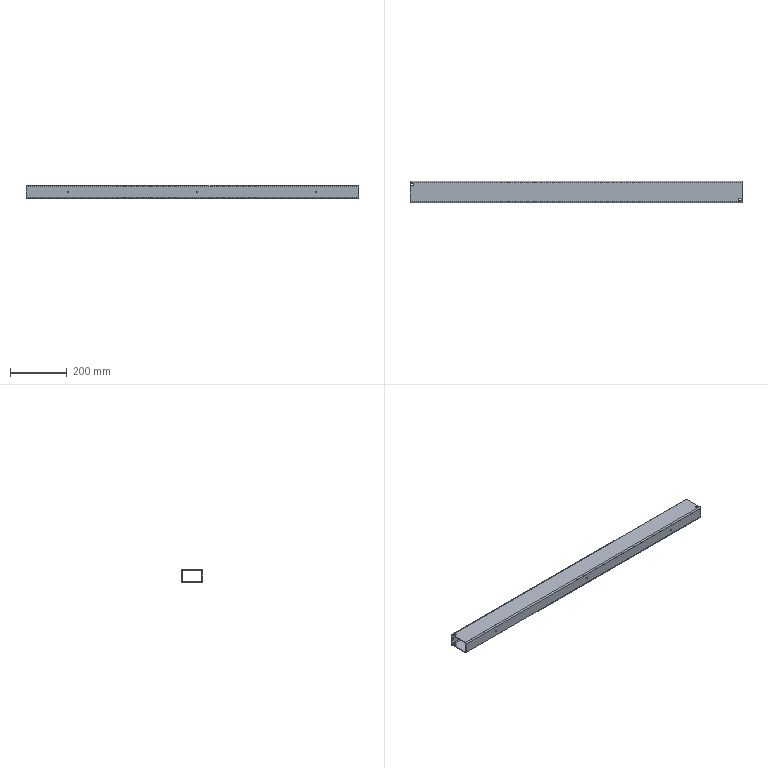Part | STEP file | [03]-3 | 1 solid | 42 faces | box 1175 x 75 x 45 mm | volume 605779 mm3 | cylinder 32 | plane 10 | commonest cylinder face diameters 10 x12 4 x6 12 x6 4.6 x4 9.2 x4
STEP:
#1=CARTESIAN_POINT('',(149.5,0.,20.5));
#2=VERTEX_POINT('',#1);
#3=CARTESIAN_POINT('',(149.5,0.,24.5));
#4=VERTEX_POINT('',#3);
#5=CARTESIAN_POINT('',(149.5,0.,22.5));
#6=DIRECTION('',(0.,1.,0.));
#7=DIRECTION('',(0.,0.,1.));
#8=AXIS2_PLACEMENT_3D('',#5,#6,#7);
#9=CIRCLE('',#8,2.);
#10=EDGE_CURVE('',#2,#4,#9,.T.);
#11=ORIENTED_EDGE('',*,*,#10,.F.);
#12=CARTESIAN_POINT('',(149.5,2.3,20.5));
#13=VERTEX_POINT('',#12);
#14=CARTESIAN_POINT('',(149.5,0.,20.5));
#15=DIRECTION('',(0.,1.,0.));
#16=VECTOR('',#15,1000.);
#17=LINE('',#14,#16);
#18=EDGE_CURVE('',#2,#13,#17,.T.);
#19=ORIENTED_EDGE('',*,*,#18,.T.);
#20=CARTESIAN_POINT('',(149.5,2.3,24.5));
#21=VERTEX_POINT('',#20);
#22=CARTESIAN_POINT('',(149.5,2.3,22.5));
#23=DIRECTION('',(0.,-1.,0.));
#24=DIRECTION('',(0.,0.,-1.));
#25=AXIS2_PLACEMENT_3D('',#22,#23,#24);
#26=CIRCLE('',#25,2.);
#27=EDGE_CURVE('',#21,#13,#26,.T.);
#28=ORIENTED_EDGE('',*,*,#27,.F.);
#29=CARTESIAN_POINT('',(149.5,0.,24.5));
#30=DIRECTION('',(0.,1.,0.));
#31=VECTOR('',#30,1000.);
#32=LINE('',#29,#31);
#33=EDGE_CURVE('',#4,#21,#32,.T.);
#34=ORIENTED_EDGE('',*,*,#33,.F.);
#35=EDGE_LOOP('',(#11,#19,#28,#34));
#36=FACE_OUTER_BOUND('',#35,.T.);
#37=CARTESIAN_POINT('',(149.5,0.,22.5));
#38=DIRECTION('',(0.,1.,0.));
#39=DIRECTION('',(0.,0.,1.));
#40=AXIS2_PLACEMENT_3D('',#37,#38,#39);
#41=CYLINDRICAL_SURFACE('',#40,2.);
#42=ADVANCED_FACE('',(#36),#41,.F.);
#43=CARTESIAN_POINT('',(604.5,0.,20.5));
#44=VERTEX_POINT('',#43);
#45=CARTESIAN_POINT('',(604.5,0.,24.5));
#46=VERTEX_POINT('',#45);
#47=CARTESIAN_POINT('',(604.5,0.,22.5));
#48=DIRECTION('',(0.,1.,0.));
#49=DIRECTION('',(0.,0.,1.));
#50=AXIS2_PLACEMENT_3D('',#47,#48,#49);
#51=CIRCLE('',#50,2.);
#52=EDGE_CURVE('',#44,#46,#51,.T.);
#53=ORIENTED_EDGE('',*,*,#52,.F.);
#54=CARTESIAN_POINT('',(604.5,2.3,20.5));
#55=VERTEX_POINT('',#54);
#56=CARTESIAN_POINT('',(604.5,0.,20.5));
#57=DIRECTION('',(0.,1.,0.));
#58=VECTOR('',#57,1000.);
#59=LINE('',#56,#58);
#60=EDGE_CURVE('',#44,#55,#59,.T.);
#61=ORIENTED_EDGE('',*,*,#60,.T.);
#62=CARTESIAN_POINT('',(604.5,2.3,24.5));
#63=VERTEX_POINT('',#62);
#64=CARTESIAN_POINT('',(604.5,2.3,22.5));
#65=DIRECTION('',(0.,-1.,0.));
#66=DIRECTION('',(0.,0.,-1.));
#67=AXIS2_PLACEMENT_3D('',#64,#65,#66);
#68=CIRCLE('',#67,2.);
#69=EDGE_CURVE('',#63,#55,#68,.T.);
#70=ORIENTED_EDGE('',*,*,#69,.F.);
#71=CARTESIAN_POINT('',(604.5,0.,24.5));
#72=DIRECTION('',(0.,1.,0.));
#73=VECTOR('',#72,1000.);
#74=LINE('',#71,#73);
#75=EDGE_CURVE('',#46,#63,#74,.T.);
#76=ORIENTED_EDGE('',*,*,#75,.F.);
#77=EDGE_LOOP('',(#53,#61,#70,#76));
#78=FACE_OUTER_BOUND('',#77,.T.);
#79=CARTESIAN_POINT('',(604.5,0.,22.5));
#80=DIRECTION('',(0.,1.,0.));
#81=DIRECTION('',(0.,0.,1.));
#82=AXIS2_PLACEMENT_3D('',#79,#80,#81);
#83=CYLINDRICAL_SURFACE('',#82,2.);
#84=ADVANCED_FACE('',(#78),#83,.F.);
#85=CARTESIAN_POINT('',(1024.5,0.,20.5));
#86=VERTEX_POINT('',#85);
#87=CARTESIAN_POINT('',(1024.5,0.,24.5));
#88=VERTEX_POINT('',#87);
#89=CARTESIAN_POINT('',(1024.5,0.,22.5));
#90=DIRECTION('',(0.,1.,0.));
#91=DIRECTION('',(0.,0.,1.));
#92=AXIS2_PLACEMENT_3D('',#89,#90,#91);
#93=CIRCLE('',#92,2.);
#94=EDGE_CURVE('',#86,#88,#93,.T.);
#95=ORIENTED_EDGE('',*,*,#94,.F.);
#96=CARTESIAN_POINT('',(1024.5,2.3,20.5));
#97=VERTEX_POINT('',#96);
#98=CARTESIAN_POINT('',(1024.5,0.,20.5));
#99=DIRECTION('',(0.,1.,0.));
#100=VECTOR('',#99,1000.);
#101=LINE('',#98,#100);
#102=EDGE_CURVE('',#86,#97,#101,.T.);
#103=ORIENTED_EDGE('',*,*,#102,.T.);
#104=CARTESIAN_POINT('',(1024.5,2.3,24.5));
#105=VERTEX_POINT('',#104);
#106=CARTESIAN_POINT('',(1024.5,2.3,22.5));
#107=DIRECTION('',(0.,-1.,0.));
#108=DIRECTION('',(0.,0.,-1.));
#109=AXIS2_PLACEMENT_3D('',#106,#107,#108);
#110=CIRCLE('',#109,2.);
#111=EDGE_CURVE('',#105,#97,#110,.T.);
#112=ORIENTED_EDGE('',*,*,#111,.F.);
#113=CARTESIAN_POINT('',(1024.5,0.,24.5));
#114=DIRECTION('',(0.,1.,0.));
#115=VECTOR('',#114,1000.);
#116=LINE('',#113,#115);
#117=EDGE_CURVE('',#88,#105,#116,.T.);
#118=ORIENTED_EDGE('',*,*,#117,.F.);
#119=EDGE_LOOP('',(#95,#103,#112,#118));
#120=FACE_OUTER_BOUND('',#119,.T.);
#121=CARTESIAN_POINT('',(1024.5,0.,22.5));
#122=DIRECTION('',(0.,1.,0.));
#123=DIRECTION('',(0.,0.,1.));
#124=AXIS2_PLACEMENT_3D('',#121,#122,#123);
#125=CYLINDRICAL_SURFACE('',#124,2.);
#126=ADVANCED_FACE('',(#120),#125,.F.);
#127=CARTESIAN_POINT('',(1167.5,75.,27.5));
#128=VERTEX_POINT('',#127);
#129=CARTESIAN_POINT('',(1167.5,75.,17.5));
#130=VERTEX_POINT('',#129);
#131=CARTESIAN_POINT('',(1167.5,75.,22.5));
#132=DIRECTION('',(0.,-1.,0.));
#133=DIRECTION('',(0.,0.,-1.));
#134=AXIS2_PLACEMENT_3D('',#131,#132,#133);
#135=CIRCLE('',#134,5.);
#136=EDGE_CURVE('',#128,#130,#135,.T.);
#137=ORIENTED_EDGE('',*,*,#136,.F.);
#138=CARTESIAN_POINT('',(1167.5,72.7,27.5));
#139=VERTEX_POINT('',#138);
#140=CARTESIAN_POINT('',(1167.5,75.,27.5));
#141=DIRECTION('',(0.,-1.,0.));
#142=VECTOR('',#141,1000.);
#143=LINE('',#140,#142);
#144=EDGE_CURVE('',#128,#139,#143,.T.);
#145=ORIENTED_EDGE('',*,*,#144,.T.);
#146=CARTESIAN_POINT('',(1167.5,72.7,17.5));
#147=VERTEX_POINT('',#146);
#148=CARTESIAN_POINT('',(1167.5,72.7,22.5));
#149=DIRECTION('',(0.,1.,0.));
#150=DIRECTION('',(0.,0.,1.));
#151=AXIS2_PLACEMENT_3D('',#148,#149,#150);
#152=CIRCLE('',#151,5.);
#153=EDGE_CURVE('',#147,#139,#152,.T.);
#154=ORIENTED_EDGE('',*,*,#153,.F.);
#155=CARTESIAN_POINT('',(1167.5,75.,17.5));
#156=DIRECTION('',(0.,-1.,0.));
#157=VECTOR('',#156,1000.);
#158=LINE('',#155,#157);
#159=EDGE_CURVE('',#130,#147,#158,.T.);
#160=ORIENTED_EDGE('',*,*,#159,.F.);
#161=EDGE_LOOP('',(#137,#145,#154,#160));
#162=FACE_OUTER_BOUND('',#161,.T.);
#163=CARTESIAN_POINT('',(1167.5,75.,22.5));
#164=DIRECTION('',(0.,-1.,0.));
#165=DIRECTION('',(0.,0.,-1.));
#166=AXIS2_PLACEMENT_3D('',#163,#164,#165);
#167=CYLINDRICAL_SURFACE('',#166,5.);
#168=ADVANCED_FACE('',(#162),#167,.F.);
#169=CARTESIAN_POINT('',(6.5,75.,27.5));
#170=VERTEX_POINT('',#169);
#171=CARTESIAN_POINT('',(6.5,75.,17.5));
#172=VERTEX_POINT('',#171);
#173=CARTESIAN_POINT('',(6.5,75.,22.5));
#174=DIRECTION('',(0.,-1.,0.));
#175=DIRECTION('',(0.,0.,-1.));
#176=AXIS2_PLACEMENT_3D('',#173,#174,#175);
#177=CIRCLE('',#176,5.);
#178=EDGE_CURVE('',#170,#172,#177,.T.);
#179=ORIENTED_EDGE('',*,*,#178,.F.);
#180=CARTESIAN_POINT('',(6.5,72.7,27.5));
#181=VERTEX_POINT('',#180);
#182=CARTESIAN_POINT('',(6.5,75.,27.5));
#183=DIRECTION('',(0.,-1.,0.));
#184=VECTOR('',#183,1000.);
#185=LINE('',#182,#184);
#186=EDGE_CURVE('',#170,#181,#185,.T.);
#187=ORIENTED_EDGE('',*,*,#186,.T.);
#188=CARTESIAN_POINT('',(6.5,72.7,17.5));
#189=VERTEX_POINT('',#188);
#190=CARTESIAN_POINT('',(6.5,72.7,22.5));
#191=DIRECTION('',(0.,1.,0.));
#192=DIRECTION('',(0.,0.,1.));
#193=AXIS2_PLACEMENT_3D('',#190,#191,#192);
#194=CIRCLE('',#193,5.);
#195=EDGE_CURVE('',#189,#181,#194,.T.);
#196=ORIENTED_EDGE('',*,*,#195,.F.);
#197=CARTESIAN_POINT('',(6.5,75.,17.5));
#198=DIRECTION('',(0.,-1.,0.));
#199=VECTOR('',#198,1000.);
#200=LINE('',#197,#199);
#201=EDGE_CURVE('',#172,#189,#200,.T.);
#202=ORIENTED_EDGE('',*,*,#201,.F.);
#203=EDGE_LOOP('',(#179,#187,#196,#202));
#204=FACE_OUTER_BOUND('',#203,.T.);
#205=CARTESIAN_POINT('',(6.5,75.,22.5));
#206=DIRECTION('',(0.,-1.,0.));
#207=DIRECTION('',(0.,0.,-1.));
#208=AXIS2_PLACEMENT_3D('',#205,#206,#207);
#209=CYLINDRICAL_SURFACE('',#208,5.);
#210=ADVANCED_FACE('',(#204),#209,.F.);
#211=CARTESIAN_POINT('',(1166.5,15.5,42.7));
#212=VERTEX_POINT('',#211);
#213=CARTESIAN_POINT('',(1166.5,5.5,42.7));
#214=VERTEX_POINT('',#213);
#215=CARTESIAN_POINT('',(1166.5,10.5,42.7));
#216=DIRECTION('',(0.,0.,1.));
#217=DIRECTION('',(0.,-1.,0.));
#218=AXIS2_PLACEMENT_3D('',#215,#216,#217);
#219=CIRCLE('',#218,5.);
#220=EDGE_CURVE('',#212,#214,#219,.T.);
#221=ORIENTED_EDGE('',*,*,#220,.F.);
#222=CARTESIAN_POINT('',(1166.5,15.5,45.));
#223=VERTEX_POINT('',#222);
#224=CARTESIAN_POINT('',(1166.5,15.5,42.7));
#225=DIRECTION('',(0.,0.,1.));
#226=VECTOR('',#225,1000.);
#227=LINE('',#224,#226);
#228=EDGE_CURVE('',#212,#223,#227,.T.);
#229=ORIENTED_EDGE('',*,*,#228,.T.);
#230=CARTESIAN_POINT('',(1166.5,5.5,45.));
#231=VERTEX_POINT('',#230);
#232=CARTESIAN_POINT('',(1166.5,10.5,45.));
#233=DIRECTION('',(0.,0.,-1.));
#234=DIRECTION('',(0.,1.,0.));
#235=AXIS2_PLACEMENT_3D('',#232,#233,#234);
#236=CIRCLE('',#235,5.);
#237=EDGE_CURVE('',#231,#223,#236,.T.);
#238=ORIENTED_EDGE('',*,*,#237,.F.);
#239=CARTESIAN_POINT('',(1166.5,5.5,42.7));
#240=DIRECTION('',(0.,0.,1.));
#241=VECTOR('',#240,1000.);
#242=LINE('',#239,#241);
#243=EDGE_CURVE('',#214,#231,#242,.T.);
#244=ORIENTED_EDGE('',*,*,#243,.F.);
#245=EDGE_LOOP('',(#221,#229,#238,#244));
#246=FACE_OUTER_BOUND('',#245,.T.);
#247=CARTESIAN_POINT('',(1166.5,10.5,42.7));
#248=DIRECTION('',(0.,0.,1.));
#249=DIRECTION('',(0.,-1.,0.));
#250=AXIS2_PLACEMENT_3D('',#247,#248,#249);
#251=CYLINDRICAL_SURFACE('',#250,5.);
#252=ADVANCED_FACE('',(#246),#251,.F.);
#253=CARTESIAN_POINT('',(7.5,59.5,2.3));
#254=VERTEX_POINT('',#253);
#255=CARTESIAN_POINT('',(7.5,69.5,2.3));
#256=VERTEX_POINT('',#255);
#257=CARTESIAN_POINT('',(7.5,64.5,2.3));
#258=DIRECTION('',(0.,0.,-1.));
#259=DIRECTION('',(0.,1.,0.));
#260=AXIS2_PLACEMENT_3D('',#257,#258,#259);
#261=CIRCLE('',#260,5.);
#262=EDGE_CURVE('',#254,#256,#261,.T.);
#263=ORIENTED_EDGE('',*,*,#262,.F.);
#264=CARTESIAN_POINT('',(7.5,59.5,0.));
#265=VERTEX_POINT('',#264);
#266=CARTESIAN_POINT('',(7.5,59.5,2.3));
#267=DIRECTION('',(0.,0.,-1.));
#268=VECTOR('',#267,1000.);
#269=LINE('',#266,#268);
#270=EDGE_CURVE('',#254,#265,#269,.T.);
#271=ORIENTED_EDGE('',*,*,#270,.T.);
#272=CARTESIAN_POINT('',(7.5,69.5,0.));
#273=VERTEX_POINT('',#272);
#274=CARTESIAN_POINT('',(7.5,64.5,0.));
#275=DIRECTION('',(0.,0.,1.));
#276=DIRECTION('',(0.,-1.,0.));
#277=AXIS2_PLACEMENT_3D('',#274,#275,#276);
#278=CIRCLE('',#277,5.);
#279=EDGE_CURVE('',#273,#265,#278,.T.);
#280=ORIENTED_EDGE('',*,*,#279,.F.);
#281=CARTESIAN_POINT('',(7.5,69.5,2.3));
#282=DIRECTION('',(0.,0.,-1.));
#283=VECTOR('',#282,1000.);
#284=LINE('',#281,#283);
#285=EDGE_CURVE('',#256,#273,#284,.T.);
#286=ORIENTED_EDGE('',*,*,#285,.F.);
#287=EDGE_LOOP('',(#263,#271,#280,#286));
#288=FACE_OUTER_BOUND('',#287,.T.);
#289=CARTESIAN_POINT('',(7.5,64.5,2.3));
#290=DIRECTION('',(0.,0.,-1.));
#291=DIRECTION('',(0.,1.,0.));
#292=AXIS2_PLACEMENT_3D('',#289,#290,#291);
#293=CYLINDRICAL_SURFACE('',#292,5.);
#294=ADVANCED_FACE('',(#288),#293,.F.);
#295=CARTESIAN_POINT('',(1024.5,51.,0.));
#296=VERTEX_POINT('',#295);
#297=CARTESIAN_POINT('',(1024.5,39.,0.));
#298=VERTEX_POINT('',#297);
#299=CARTESIAN_POINT('',(1024.5,45.,0.));
#300=DIRECTION('',(0.,0.,1.));
#301=DIRECTION('',(0.,-1.,0.));
#302=AXIS2_PLACEMENT_3D('',#299,#300,#301);
#303=CIRCLE('',#302,6.);
#304=EDGE_CURVE('',#296,#298,#303,.T.);
#305=ORIENTED_EDGE('',*,*,#304,.F.);
#306=CARTESIAN_POINT('',(1024.5,51.,2.3));
#307=VERTEX_POINT('',#306);
#308=CARTESIAN_POINT('',(1024.5,51.,0.));
#309=DIRECTION('',(0.,0.,1.));
#310=VECTOR('',#309,1000.);
#311=LINE('',#308,#310);
#312=EDGE_CURVE('',#296,#307,#311,.T.);
#313=ORIENTED_EDGE('',*,*,#312,.T.);
#314=CARTESIAN_POINT('',(1024.5,39.,2.3));
#315=VERTEX_POINT('',#314);
#316=CARTESIAN_POINT('',(1024.5,45.,2.3));
#317=DIRECTION('',(0.,0.,-1.));
#318=DIRECTION('',(0.,1.,0.));
#319=AXIS2_PLACEMENT_3D('',#316,#317,#318);
#320=CIRCLE('',#319,6.);
#321=EDGE_CURVE('',#315,#307,#320,.T.);
#322=ORIENTED_EDGE('',*,*,#321,.F.);
#323=CARTESIAN_POINT('',(1024.5,39.,0.));
#324=DIRECTION('',(0.,0.,1.));
#325=VECTOR('',#324,1000.);
#326=LINE('',#323,#325);
#327=EDGE_CURVE('',#298,#315,#326,.T.);
#328=ORIENTED_EDGE('',*,*,#327,.F.);
#329=EDGE_LOOP('',(#305,#313,#322,#328));
#330=FACE_OUTER_BOUND('',#329,.T.);
#331=CARTESIAN_POINT('',(1024.5,45.,0.));
#332=DIRECTION('',(0.,0.,1.));
#333=DIRECTION('',(0.,-1.,0.));
#334=AXIS2_PLACEMENT_3D('',#331,#332,#333);
#335=CYLINDRICAL_SURFACE('',#334,6.);
#336=ADVANCED_FACE('',(#330),#335,.F.);
#337=CARTESIAN_POINT('',(749.5,51.,0.));
#338=VERTEX_POINT('',#337);
#339=CARTESIAN_POINT('',(749.5,39.,0.));
#340=VERTEX_POINT('',#339);
#341=CARTESIAN_POINT('',(749.5,45.,0.));
#342=DIRECTION('',(0.,0.,1.));
#343=DIRECTION('',(0.,-1.,0.));
#344=AXIS2_PLACEMENT_3D('',#341,#342,#343);
#345=CIRCLE('',#344,6.);
#346=EDGE_CURVE('',#338,#340,#345,.T.);
#347=ORIENTED_EDGE('',*,*,#346,.F.);
#348=CARTESIAN_POINT('',(749.5,51.,2.3));
#349=VERTEX_POINT('',#348);
#350=CARTESIAN_POINT('',(749.5,51.,0.));
#351=DIRECTION('',(0.,0.,1.));
#352=VECTOR('',#351,1000.);
#353=LINE('',#350,#352);
#354=EDGE_CURVE('',#338,#349,#353,.T.);
#355=ORIENTED_EDGE('',*,*,#354,.T.);
#356=CARTESIAN_POINT('',(749.5,39.,2.3));
#357=VERTEX_POINT('',#356);
#358=CARTESIAN_POINT('',(749.5,45.,2.3));
#359=DIRECTION('',(0.,0.,-1.));
#360=DIRECTION('',(0.,1.,0.));
#361=AXIS2_PLACEMENT_3D('',#358,#359,#360);
#362=CIRCLE('',#361,6.);
#363=EDGE_CURVE('',#357,#349,#362,.T.);
#364=ORIENTED_EDGE('',*,*,#363,.F.);
#365=CARTESIAN_POINT('',(749.5,39.,0.));
#366=DIRECTION('',(0.,0.,1.));
#367=VECTOR('',#366,1000.);
#368=LINE('',#365,#367);
#369=EDGE_CURVE('',#340,#357,#368,.T.);
#370=ORIENTED_EDGE('',*,*,#369,.F.);
#371=EDGE_LOOP('',(#347,#355,#364,#370));
#372=FACE_OUTER_BOUND('',#371,.T.);
#373=CARTESIAN_POINT('',(749.5,45.,0.));
#374=DIRECTION('',(0.,0.,1.));
#375=DIRECTION('',(0.,-1.,0.));
#376=AXIS2_PLACEMENT_3D('',#373,#374,#375);
#377=CYLINDRICAL_SURFACE('',#376,6.);
#378=ADVANCED_FACE('',(#372),#377,.F.);
#379=CARTESIAN_POINT('',(474.5,51.,0.));
#380=VERTEX_POINT('',#379);
#381=CARTESIAN_POINT('',(474.5,39.,0.));
#382=VERTEX_POINT('',#381);
#383=CARTESIAN_POINT('',(474.5,45.,0.));
#384=DIRECTION('',(0.,0.,1.));
#385=DIRECTION('',(0.,-1.,0.));
#386=AXIS2_PLACEMENT_3D('',#383,#384,#385);
#387=CIRCLE('',#386,6.);
#388=EDGE_CURVE('',#380,#382,#387,.T.);
#389=ORIENTED_EDGE('',*,*,#388,.F.);
#390=CARTESIAN_POINT('',(474.5,51.,2.3));
#391=VERTEX_POINT('',#390);
#392=CARTESIAN_POINT('',(474.5,51.,0.));
#393=DIRECTION('',(0.,0.,1.));
#394=VECTOR('',#393,1000.);
#395=LINE('',#392,#394);
#396=EDGE_CURVE('',#380,#391,#395,.T.);
#397=ORIENTED_EDGE('',*,*,#396,.T.);
#398=CARTESIAN_POINT('',(474.5,39.,2.3));
#399=VERTEX_POINT('',#398);
#400=CARTESIAN_POINT('',(474.5,45.,2.3));
#401=DIRECTION('',(0.,0.,-1.));
#402=DIRECTION('',(0.,1.,0.));
#403=AXIS2_PLACEMENT_3D('',#400,#401,#402);
#404=CIRCLE('',#403,6.);
#405=EDGE_CURVE('',#399,#391,#404,.T.);
#406=ORIENTED_EDGE('',*,*,#405,.F.);
#407=CARTESIAN_POINT('',(474.5,39.,0.));
#408=DIRECTION('',(0.,0.,1.));
#409=VECTOR('',#408,1000.);
#410=LINE('',#407,#409);
#411=EDGE_CURVE('',#382,#399,#410,.T.);
#412=ORIENTED_EDGE('',*,*,#411,.F.);
#413=EDGE_LOOP('',(#389,#397,#406,#412));
#414=FACE_OUTER_BOUND('',#413,.T.);
#415=CARTESIAN_POINT('',(474.5,45.,0.));
#416=DIRECTION('',(0.,0.,1.));
#417=DIRECTION('',(0.,-1.,0.));
#418=AXIS2_PLACEMENT_3D('',#415,#416,#417);
#419=CYLINDRICAL_SURFACE('',#418,6.);
#420=ADVANCED_FACE('',(#414),#419,.F.);
#421=CARTESIAN_POINT('',(7.5,59.5,45.));
#422=VERTEX_POINT('',#421);
#423=CARTESIAN_POINT('',(7.5,69.5,45.));
#424=VERTEX_POINT('',#423);
#425=CARTESIAN_POINT('',(7.5,64.5,45.));
#426=DIRECTION('',(0.,0.,-1.));
#427=DIRECTION('',(0.,1.,0.));
#428=AXIS2_PLACEMENT_3D('',#425,#426,#427);
#429=CIRCLE('',#428,5.);
#430=EDGE_CURVE('',#422,#424,#429,.T.);
#431=ORIENTED_EDGE('',*,*,#430,.F.);
#432=CARTESIAN_POINT('',(7.5,59.5,42.7));
#433=VERTEX_POINT('',#432);
#434=CARTESIAN_POINT('',(7.5,59.5,45.));
#435=DIRECTION('',(0.,0.,-1.));
#436=VECTOR('',#435,1000.);
#437=LINE('',#434,#436);
#438=EDGE_CURVE('',#422,#433,#437,.T.);
#439=ORIENTED_EDGE('',*,*,#438,.T.);
#440=CARTESIAN_POINT('',(7.5,69.5,42.7));
#441=VERTEX_POINT('',#440);
#442=CARTESIAN_POINT('',(7.5,64.5,42.7));
#443=DIRECTION('',(0.,0.,1.));
#444=DIRECTION('',(0.,-1.,0.));
#445=AXIS2_PLACEMENT_3D('',#442,#443,#444);
#446=CIRCLE('',#445,5.);
#447=EDGE_CURVE('',#441,#433,#446,.T.);
#448=ORIENTED_EDGE('',*,*,#447,.F.);
#449=CARTESIAN_POINT('',(7.5,69.5,45.));
#450=DIRECTION('',(0.,0.,-1.));
#451=VECTOR('',#450,1000.);
#452=LINE('',#449,#451);
#453=EDGE_CURVE('',#424,#441,#452,.T.);
#454=ORIENTED_EDGE('',*,*,#453,.F.);
#455=EDGE_LOOP('',(#431,#439,#448,#454));
#456=FACE_OUTER_BOUND('',#455,.T.);
#457=CARTESIAN_POINT('',(7.5,64.5,45.));
#458=DIRECTION('',(0.,0.,-1.));
#459=DIRECTION('',(0.,1.,0.));
#460=AXIS2_PLACEMENT_3D('',#457,#458,#459);
#461=CYLINDRICAL_SURFACE('',#460,5.);
#462=ADVANCED_FACE('',(#456),#461,.F.);
#463=CARTESIAN_POINT('',(1166.5,15.5,0.));
#464=VERTEX_POINT('',#463);
#465=CARTESIAN_POINT('',(1166.5,5.5,0.));
#466=VERTEX_POINT('',#465);
#467=CARTESIAN_POINT('',(1166.5,10.5,0.));
#468=DIRECTION('',(0.,0.,1.));
#469=DIRECTION('',(0.,-1.,0.));
#470=AXIS2_PLACEMENT_3D('',#467,#468,#469);
#471=CIRCLE('',#470,5.);
#472=EDGE_CURVE('',#464,#466,#471,.T.);
#473=ORIENTED_EDGE('',*,*,#472,.F.);
#474=CARTESIAN_POINT('',(1166.5,15.5,2.3));
#475=VERTEX_POINT('',#474);
#476=CARTESIAN_POINT('',(1166.5,15.5,0.));
#477=DIRECTION('',(0.,0.,1.));
#478=VECTOR('',#477,1000.);
#479=LINE('',#476,#478);
#480=EDGE_CURVE('',#464,#475,#479,.T.);
#481=ORIENTED_EDGE('',*,*,#480,.T.);
#482=CARTESIAN_POINT('',(1166.5,5.5,2.3));
#483=VERTEX_POINT('',#482);
#484=CARTESIAN_POINT('',(1166.5,10.5,2.3));
#485=DIRECTION('',(0.,0.,-1.));
#486=DIRECTION('',(0.,1.,0.));
#487=AXIS2_PLACEMENT_3D('',#484,#485,#486);
#488=CIRCLE('',#487,5.);
#489=EDGE_CURVE('',#483,#475,#488,.T.);
#490=ORIENTED_EDGE('',*,*,#489,.F.);
#491=CARTESIAN_POINT('',(1166.5,5.5,0.));
#492=DIRECTION('',(0.,0.,1.));
#493=VECTOR('',#492,1000.);
#494=LINE('',#491,#493);
#495=EDGE_CURVE('',#466,#483,#494,.T.);
#496=ORIENTED_EDGE('',*,*,#495,.F.);
#497=EDGE_LOOP('',(#473,#481,#490,#496));
#498=FACE_OUTER_BOUND('',#497,.T.);
#499=CARTESIAN_POINT('',(1166.5,10.5,0.));
#500=DIRECTION('',(0.,0.,1.));
#501=DIRECTION('',(0.,-1.,0.));
#502=AXIS2_PLACEMENT_3D('',#499,#500,#501);
#503=CYLINDRICAL_SURFACE('',#502,5.);
#504=ADVANCED_FACE('',(#498),#503,.F.);
#505=CARTESIAN_POINT('',(1174.5,4.6,0.));
#506=VERTEX_POINT('',#505);
#507=CARTESIAN_POINT('',(1174.5,70.4,0.));
#508=VERTEX_POINT('',#507);
#509=CARTESIAN_POINT('',(1174.5,4.6,0.));
#510=DIRECTION('',(0.,1.,0.));
#511=VECTOR('',#510,1000.);
#512=LINE('',#509,#511);
#513=EDGE_CURVE('',#506,#508,#512,.T.);
#514=ORIENTED_EDGE('',*,*,#513,.T.);
#515=CARTESIAN_POINT('',(1174.5,75.,4.6));
#516=VERTEX_POINT('',#515);
#517=CARTESIAN_POINT('',(1174.5,70.4,4.6));
#518=DIRECTION('',(1.,0.,0.));
#519=DIRECTION('',(0.,0.,-1.));
#520=AXIS2_PLACEMENT_3D('',#517,#518,#519);
#521=CIRCLE('',#520,4.6);
#522=EDGE_CURVE('',#508,#516,#521,.T.);
#523=ORIENTED_EDGE('',*,*,#522,.T.);
#524=CARTESIAN_POINT('',(1174.5,75.,40.4));
#525=VERTEX_POINT('',#524);
#526=CARTESIAN_POINT('',(1174.5,75.,4.6));
#527=DIRECTION('',(0.,0.,1.));
#528=VECTOR('',#527,1000.);
#529=LINE('',#526,#528);
#530=EDGE_CURVE('',#516,#525,#529,.T.);
#531=ORIENTED_EDGE('',*,*,#530,.T.);
#532=CARTESIAN_POINT('',(1174.5,70.4,45.));
#533=VERTEX_POINT('',#532);
#534=CARTESIAN_POINT('',(1174.5,70.4,40.4));
#535=DIRECTION('',(1.,0.,0.));
#536=DIRECTION('',(0.,0.,-1.));
#537=AXIS2_PLACEMENT_3D('',#534,#535,#536);
#538=CIRCLE('',#537,4.6);
#539=EDGE_CURVE('',#525,#533,#538,.T.);
#540=ORIENTED_EDGE('',*,*,#539,.T.);
#541=CARTESIAN_POINT('',(1174.5,4.6,45.));
#542=VERTEX_POINT('',#541);
#543=CARTESIAN_POINT('',(1174.5,70.4,45.));
#544=DIRECTION('',(0.,-1.,0.));
#545=VECTOR('',#544,1000.);
#546=LINE('',#543,#545);
#547=EDGE_CURVE('',#533,#542,#546,.T.);
#548=ORIENTED_EDGE('',*,*,#547,.T.);
#549=CARTESIAN_POINT('',(1174.5,0.,40.4));
#550=VERTEX_POINT('',#549);
#551=CARTESIAN_POINT('',(1174.5,4.6,40.4));
#552=DIRECTION('',(1.,0.,0.));
#553=DIRECTION('',(0.,0.,-1.));
#554=AXIS2_PLACEMENT_3D('',#551,#552,#553);
#555=CIRCLE('',#554,4.6);
#556=EDGE_CURVE('',#542,#550,#555,.T.);
#557=ORIENTED_EDGE('',*,*,#556,.T.);
#558=CARTESIAN_POINT('',(1174.5,0.,4.6));
#559=VERTEX_POINT('',#558);
#560=CARTESIAN_POINT('',(1174.5,0.,40.4));
#561=DIRECTION('',(0.,0.,-1.));
#562=VECTOR('',#561,1000.);
#563=LINE('',#560,#562);
#564=EDGE_CURVE('',#550,#559,#563,.T.);
#565=ORIENTED_EDGE('',*,*,#564,.T.);
#566=CARTESIAN_POINT('',(1174.5,4.6,4.6));
#567=DIRECTION('',(1.,0.,0.));
#568=DIRECTION('',(0.,0.,-1.));
#569=AXIS2_PLACEMENT_3D('',#566,#567,#568);
#570=CIRCLE('',#569,4.6);
#571=EDGE_CURVE('',#559,#506,#570,.T.);
#572=ORIENTED_EDGE('',*,*,#571,.T.);
#573=EDGE_LOOP('',(#514,#523,#531,#540,#548,#557,#565,#572));
#574=FACE_OUTER_BOUND('',#573,.T.);
#575=CARTESIAN_POINT('',(1174.5,4.6,2.3));
#576=VERTEX_POINT('',#575);
#577=CARTESIAN_POINT('',(1174.5,70.4,2.3));
#578=VERTEX_POINT('',#577);
#579=CARTESIAN_POINT('',(1174.5,4.6,2.3));
#580=DIRECTION('',(0.,1.,0.));
#581=VECTOR('',#580,1000.);
#582=LINE('',#579,#581);
#583=EDGE_CURVE('',#576,#578,#582,.T.);
#584=ORIENTED_EDGE('',*,*,#583,.F.);
#585=CARTESIAN_POINT('',(1174.5,2.3,4.6));
#586=VERTEX_POINT('',#585);
#587=CARTESIAN_POINT('',(1174.5,4.6,4.6));
#588=DIRECTION('',(1.,0.,0.));
#589=DIRECTION('',(0.,-1.,0.));
#590=AXIS2_PLACEMENT_3D('',#587,#588,#589);
#591=CIRCLE('',#590,2.3);
#592=EDGE_CURVE('',#586,#576,#591,.T.);
#593=ORIENTED_EDGE('',*,*,#592,.F.);
#594=CARTESIAN_POINT('',(1174.5,2.3,40.4));
#595=VERTEX_POINT('',#594);
#596=CARTESIAN_POINT('',(1174.5,2.3,40.4));
#597=DIRECTION('',(0.,0.,-1.));
#598=VECTOR('',#597,1000.);
#599=LINE('',#596,#598);
#600=EDGE_CURVE('',#595,#586,#599,.T.);
#601=ORIENTED_EDGE('',*,*,#600,.F.);
#602=CARTESIAN_POINT('',(1174.5,4.6,42.7));
#603=VERTEX_POINT('',#602);
#604=CARTESIAN_POINT('',(1174.5,4.6,40.4));
#605=DIRECTION('',(1.,0.,0.));
#606=DIRECTION('',(0.,-1.,0.));
#607=AXIS2_PLACEMENT_3D('',#604,#605,#606);
#608=CIRCLE('',#607,2.3);
#609=EDGE_CURVE('',#603,#595,#608,.T.);
#610=ORIENTED_EDGE('',*,*,#609,.F.);
#611=CARTESIAN_POINT('',(1174.5,70.4,42.7));
#612=VERTEX_POINT('',#611);
#613=CARTESIAN_POINT('',(1174.5,70.4,42.7));
#614=DIRECTION('',(0.,-1.,0.));
#615=VECTOR('',#614,1000.);
#616=LINE('',#613,#615);
#617=EDGE_CURVE('',#612,#603,#616,.T.);
#618=ORIENTED_EDGE('',*,*,#617,.F.);
#619=CARTESIAN_POINT('',(1174.5,72.7,40.4));
#620=VERTEX_POINT('',#619);
#621=CARTESIAN_POINT('',(1174.5,70.4,40.4));
#622=DIRECTION('',(1.,0.,0.));
#623=DIRECTION('',(0.,-1.,0.));
#624=AXIS2_PLACEMENT_3D('',#621,#622,#623);
#625=CIRCLE('',#624,2.3);
#626=EDGE_CURVE('',#620,#612,#625,.T.);
#627=ORIENTED_EDGE('',*,*,#626,.F.);
#628=CARTESIAN_POINT('',(1174.5,72.7,4.6));
#629=VERTEX_POINT('',#628);
#630=CARTESIAN_POINT('',(1174.5,72.7,4.6));
#631=DIRECTION('',(0.,0.,1.));
#632=VECTOR('',#631,1000.);
#633=LINE('',#630,#632);
#634=EDGE_CURVE('',#629,#620,#633,.T.);
#635=ORIENTED_EDGE('',*,*,#634,.F.);
#636=CARTESIAN_POINT('',(1174.5,70.4,4.6));
#637=DIRECTION('',(1.,0.,0.));
#638=DIRECTION('',(0.,-1.,0.));
#639=AXIS2_PLACEMENT_3D('',#636,#637,#638);
#640=CIRCLE('',#639,2.3);
#641=EDGE_CURVE('',#578,#629,#640,.T.);
#642=ORIENTED_EDGE('',*,*,#641,.F.);
#643=EDGE_LOOP('',(#584,#593,#601,#610,#618,#627,#635,#642));
#644=FACE_BOUND('',#643,.T.);
#645=CARTESIAN_POINT('',(1174.5,70.4,4.6));
#646=DIRECTION('',(1.,0.,0.));
#647=DIRECTION('',(0.,0.,-1.));
#648=AXIS2_PLACEMENT_3D('',#645,#646,#647);
#649=PLANE('',#648);
#650=ADVANCED_FACE('',(#574,#644),#649,.T.);
#651=CARTESIAN_POINT('',(-0.5,4.6,0.));
#652=VERTEX_POINT('',#651);
#653=CARTESIAN_POINT('',(-0.5,70.4,0.));
#654=VERTEX_POINT('',#653);
#655=CARTESIAN_POINT('',(-0.5,4.6,0.));
#656=DIRECTION('',(0.,1.,0.));
#657=VECTOR('',#656,1000.);
#658=LINE('',#655,#657);
#659=EDGE_CURVE('',#652,#654,#658,.T.);
#660=ORIENTED_EDGE('',*,*,#659,.F.);
#661=CARTESIAN_POINT('',(-0.5,0.,4.6));
#662=VERTEX_POINT('',#661);
#663=CARTESIAN_POINT('',(-0.5,4.6,4.6));
#664=DIRECTION('',(1.,0.,0.));
#665=DIRECTION('',(0.,0.,-1.));
#666=AXIS2_PLACEMENT_3D('',#663,#664,#665);
#667=CIRCLE('',#666,4.6);
#668=EDGE_CURVE('',#662,#652,#667,.T.);
#669=ORIENTED_EDGE('',*,*,#668,.F.);
#670=CARTESIAN_POINT('',(-0.5,0.,40.4));
#671=VERTEX_POINT('',#670);
#672=CARTESIAN_POINT('',(-0.5,0.,40.4));
#673=DIRECTION('',(0.,0.,-1.));
#674=VECTOR('',#673,1000.);
#675=LINE('',#672,#674);
#676=EDGE_CURVE('',#671,#662,#675,.T.);
#677=ORIENTED_EDGE('',*,*,#676,.F.);
#678=CARTESIAN_POINT('',(-0.5,4.6,45.));
#679=VERTEX_POINT('',#678);
#680=CARTESIAN_POINT('',(-0.5,4.6,40.4));
#681=DIRECTION('',(1.,0.,0.));
#682=DIRECTION('',(0.,0.,-1.));
#683=AXIS2_PLACEMENT_3D('',#680,#681,#682);
#684=CIRCLE('',#683,4.6);
#685=EDGE_CURVE('',#679,#671,#684,.T.);
#686=ORIENTED_EDGE('',*,*,#685,.F.);
#687=CARTESIAN_POINT('',(-0.5,70.4,45.));
#688=VERTEX_POINT('',#687);
#689=CARTESIAN_POINT('',(-0.5,70.4,45.));
#690=DIRECTION('',(0.,-1.,0.));
#691=VECTOR('',#690,1000.);
#692=LINE('',#689,#691);
#693=EDGE_CURVE('',#688,#679,#692,.T.);
#694=ORIENTED_EDGE('',*,*,#693,.F.);
#695=CARTESIAN_POINT('',(-0.5,75.,40.4));
#696=VERTEX_POINT('',#695);
#697=CARTESIAN_POINT('',(-0.5,70.4,40.4));
#698=DIRECTION('',(1.,0.,0.));
#699=DIRECTION('',(0.,0.,-1.));
#700=AXIS2_PLACEMENT_3D('',#697,#698,#699);
#701=CIRCLE('',#700,4.6);
#702=EDGE_CURVE('',#696,#688,#701,.T.);
#703=ORIENTED_EDGE('',*,*,#702,.F.);
#704=CARTESIAN_POINT('',(-0.5,75.,4.6));
#705=VERTEX_POINT('',#704);
#706=CARTESIAN_POINT('',(-0.5,75.,4.6));
#707=DIRECTION('',(0.,0.,1.));
#708=VECTOR('',#707,1000.);
#709=LINE('',#706,#708);
#710=EDGE_CURVE('',#705,#696,#709,.T.);
#711=ORIENTED_EDGE('',*,*,#710,.F.);
#712=CARTESIAN_POINT('',(-0.5,70.4,4.6));
#713=DIRECTION('',(1.,0.,0.));
#714=DIRECTION('',(0.,0.,-1.));
#715=AXIS2_PLACEMENT_3D('',#712,#713,#714);
#716=CIRCLE('',#715,4.6);
#717=EDGE_CURVE('',#654,#705,#716,.T.);
#718=ORIENTED_EDGE('',*,*,#717,.F.);
#719=EDGE_LOOP('',(#660,#669,#677,#686,#694,#703,#711,#718));
#720=FACE_OUTER_BOUND('',#719,.T.);
#721=CARTESIAN_POINT('',(-0.5,2.3,4.6));
#722=VERTEX_POINT('',#721);
#723=CARTESIAN_POINT('',(-0.5,4.6,2.3));
#724=VERTEX_POINT('',#723);
#725=CARTESIAN_POINT('',(-0.5,4.6,4.6));
#726=DIRECTION('',(1.,0.,0.));
#727=DIRECTION('',(0.,-1.,0.));
#728=AXIS2_PLACEMENT_3D('',#725,#726,#727);
#729=CIRCLE('',#728,2.3);
#730=EDGE_CURVE('',#722,#724,#729,.T.);
#731=ORIENTED_EDGE('',*,*,#730,.T.);
#732=CARTESIAN_POINT('',(-0.5,70.4,2.3));
#733=VERTEX_POINT('',#732);
#734=CARTESIAN_POINT('',(-0.5,4.6,2.3));
#735=DIRECTION('',(0.,1.,0.));
#736=VECTOR('',#735,1000.);
#737=LINE('',#734,#736);
#738=EDGE_CURVE('',#724,#733,#737,.T.);
#739=ORIENTED_EDGE('',*,*,#738,.T.);
#740=CARTESIAN_POINT('',(-0.5,72.7,4.6));
#741=VERTEX_POINT('',#740);
#742=CARTESIAN_POINT('',(-0.5,70.4,4.6));
#743=DIRECTION('',(1.,0.,0.));
#744=DIRECTION('',(0.,-1.,0.));
#745=AXIS2_PLACEMENT_3D('',#742,#743,#744);
#746=CIRCLE('',#745,2.3);
#747=EDGE_CURVE('',#733,#741,#746,.T.);
#748=ORIENTED_EDGE('',*,*,#747,.T.);
#749=CARTESIAN_POINT('',(-0.5,72.7,40.4));
#750=VERTEX_POINT('',#749);
#751=CARTESIAN_POINT('',(-0.5,72.7,4.6));
#752=DIRECTION('',(0.,0.,1.));
#753=VECTOR('',#752,1000.);
#754=LINE('',#751,#753);
#755=EDGE_CURVE('',#741,#750,#754,.T.);
#756=ORIENTED_EDGE('',*,*,#755,.T.);
#757=CARTESIAN_POINT('',(-0.5,70.4,42.7));
#758=VERTEX_POINT('',#757);
#759=CARTESIAN_POINT('',(-0.5,70.4,40.4));
#760=DIRECTION('',(1.,0.,0.));
#761=DIRECTION('',(0.,-1.,0.));
#762=AXIS2_PLACEMENT_3D('',#759,#760,#761);
#763=CIRCLE('',#762,2.3);
#764=EDGE_CURVE('',#750,#758,#763,.T.);
#765=ORIENTED_EDGE('',*,*,#764,.T.);
#766=CARTESIAN_POINT('',(-0.5,4.6,42.7));
#767=VERTEX_POINT('',#766);
#768=CARTESIAN_POINT('',(-0.5,70.4,42.7));
#769=DIRECTION('',(0.,-1.,0.));
#770=VECTOR('',#769,1000.);
#771=LINE('',#768,#770);
#772=EDGE_CURVE('',#758,#767,#771,.T.);
#773=ORIENTED_EDGE('',*,*,#772,.T.);
#774=CARTESIAN_POINT('',(-0.5,2.3,40.4));
#775=VERTEX_POINT('',#774);
#776=CARTESIAN_POINT('',(-0.5,4.6,40.4));
#777=DIRECTION('',(1.,0.,0.));
#778=DIRECTION('',(0.,-1.,0.));
#779=AXIS2_PLACEMENT_3D('',#776,#777,#778);
#780=CIRCLE('',#779,2.3);
#781=EDGE_CURVE('',#767,#775,#780,.T.);
#782=ORIENTED_EDGE('',*,*,#781,.T.);
#783=CARTESIAN_POINT('',(-0.5,2.3,40.4));
#784=DIRECTION('',(0.,0.,-1.));
#785=VECTOR('',#784,1000.);
#786=LINE('',#783,#785);
#787=EDGE_CURVE('',#775,#722,#786,.T.);
#788=ORIENTED_EDGE('',*,*,#787,.T.);
#789=EDGE_LOOP('',(#731,#739,#748,#756,#765,#773,#782,#788));
#790=FACE_BOUND('',#789,.T.);
#791=CARTESIAN_POINT('',(-0.5,70.4,4.6));
#792=DIRECTION('',(1.,0.,0.));
#793=DIRECTION('',(0.,0.,-1.));
#794=AXIS2_PLACEMENT_3D('',#791,#792,#793);
#795=PLANE('',#794);
#796=ADVANCED_FACE('',(#720,#790),#795,.F.);
#797=ORIENTED_EDGE('',*,*,#279,.T.);
#798=CARTESIAN_POINT('',(7.5,64.5,0.));
#799=DIRECTION('',(0.,0.,1.));
#800=DIRECTION('',(0.,-1.,0.));
#801=AXIS2_PLACEMENT_3D('',#798,#799,#800);
#802=CIRCLE('',#801,5.);
#803=EDGE_CURVE('',#265,#273,#802,.T.);
#804=ORIENTED_EDGE('',*,*,#803,.T.);
#805=EDGE_LOOP('',(#797,#804));
#806=FACE_BOUND('',#805,.T.);
#807=CARTESIAN_POINT('',(1024.5,45.,0.));
#808=DIRECTION('',(0.,0.,1.));
#809=DIRECTION('',(0.,-1.,0.));
#810=AXIS2_PLACEMENT_3D('',#807,#808,#809);
#811=CIRCLE('',#810,6.);
#812=EDGE_CURVE('',#298,#296,#811,.T.);
#813=ORIENTED_EDGE('',*,*,#812,.T.);
#814=ORIENTED_EDGE('',*,*,#304,.T.);
#815=EDGE_LOOP('',(#813,#814));
#816=FACE_BOUND('',#815,.T.);
#817=CARTESIAN_POINT('',(749.5,45.,0.));
#818=DIRECTION('',(0.,0.,1.));
#819=DIRECTION('',(0.,-1.,0.));
#820=AXIS2_PLACEMENT_3D('',#817,#818,#819);
#821=CIRCLE('',#820,6.);
#822=EDGE_CURVE('',#340,#338,#821,.T.);
#823=ORIENTED_EDGE('',*,*,#822,.T.);
#824=ORIENTED_EDGE('',*,*,#346,.T.);
#825=EDGE_LOOP('',(#823,#824));
#826=FACE_BOUND('',#825,.T.);
#827=CARTESIAN_POINT('',(474.5,45.,0.));
#828=DIRECTION('',(0.,0.,1.));
#829=DIRECTION('',(0.,-1.,0.));
#830=AXIS2_PLACEMENT_3D('',#827,#828,#829);
#831=CIRCLE('',#830,6.);
#832=EDGE_CURVE('',#382,#380,#831,.T.);
#833=ORIENTED_EDGE('',*,*,#832,.T.);
#834=ORIENTED_EDGE('',*,*,#388,.T.);
#835=EDGE_LOOP('',(#833,#834));
#836=FACE_BOUND('',#835,.T.);
#837=CARTESIAN_POINT('',(1166.5,10.5,0.));
#838=DIRECTION('',(0.,0.,1.));
#839=DIRECTION('',(0.,-1.,0.));
#840=AXIS2_PLACEMENT_3D('',#837,#838,#839);
#841=CIRCLE('',#840,5.);
#842=EDGE_CURVE('',#466,#464,#841,.T.);
#843=ORIENTED_EDGE('',*,*,#842,.T.);
#844=ORIENTED_EDGE('',*,*,#472,.T.);
#845=EDGE_LOOP('',(#843,#844));
#846=FACE_BOUND('',#845,.T.);
#847=ORIENTED_EDGE('',*,*,#659,.T.);
#848=CARTESIAN_POINT('',(1174.5,70.4,0.));
#849=DIRECTION('',(-1.,0.,0.));
#850=VECTOR('',#849,1000.);
#851=LINE('',#848,#850);
#852=EDGE_CURVE('',#508,#654,#851,.T.);
#853=ORIENTED_EDGE('',*,*,#852,.F.);
#854=ORIENTED_EDGE('',*,*,#513,.F.);
#855=CARTESIAN_POINT('',(1174.5,4.6,0.));
#856=DIRECTION('',(-1.,0.,0.));
#857=VECTOR('',#856,1000.);
#858=LINE('',#855,#857);
#859=EDGE_CURVE('',#506,#652,#858,.T.);
#860=ORIENTED_EDGE('',*,*,#859,.T.);
#861=EDGE_LOOP('',(#847,#853,#854,#860));
#862=FACE_OUTER_BOUND('',#861,.T.);
#863=CARTESIAN_POINT('',(1174.5,4.6,0.));
#864=DIRECTION('',(0.,0.,1.));
#865=DIRECTION('',(0.,-1.,0.));
#866=AXIS2_PLACEMENT_3D('',#863,#864,#865);
#867=PLANE('',#866);
#868=ADVANCED_FACE('',(#806,#816,#826,#836,#846,#862),#867,.F.);
#869=ORIENTED_EDGE('',*,*,#717,.T.);
#870=CARTESIAN_POINT('',(1174.5,75.,4.6));
#871=DIRECTION('',(-1.,0.,0.));
#872=VECTOR('',#871,1000.);
#873=LINE('',#870,#872);
#874=EDGE_CURVE('',#516,#705,#873,.T.);
#875=ORIENTED_EDGE('',*,*,#874,.F.);
#876=ORIENTED_EDGE('',*,*,#522,.F.);
#877=ORIENTED_EDGE('',*,*,#852,.T.);
#878=EDGE_LOOP('',(#869,#875,#876,#877));
#879=FACE_OUTER_BOUND('',#878,.T.);
#880=CARTESIAN_POINT('',(1174.5,70.4,4.6));
#881=DIRECTION('',(-1.,0.,0.));
#882=DIRECTION('',(0.,0.,1.));
#883=AXIS2_PLACEMENT_3D('',#880,#881,#882);
#884=CYLINDRICAL_SURFACE('',#883,4.6);
#885=ADVANCED_FACE('',(#879),#884,.T.);
#886=CARTESIAN_POINT('',(1167.5,75.,22.5));
#887=DIRECTION('',(0.,-1.,0.));
#888=DIRECTION('',(0.,0.,-1.));
#889=AXIS2_PLACEMENT_3D('',#886,#887,#888);
#890=CIRCLE('',#889,5.);
#891=EDGE_CURVE('',#130,#128,#890,.T.);
#892=ORIENTED_EDGE('',*,*,#891,.T.);
#893=ORIENTED_EDGE('',*,*,#136,.T.);
#894=EDGE_LOOP('',(#892,#893));
#895=FACE_BOUND('',#894,.T.);
#896=CARTESIAN_POINT('',(6.5,75.,22.5));
#897=DIRECTION('',(0.,-1.,0.));
#898=DIRECTION('',(0.,0.,-1.));
#899=AXIS2_PLACEMENT_3D('',#896,#897,#898);
#900=CIRCLE('',#899,5.);
#901=EDGE_CURVE('',#172,#170,#900,.T.);
#902=ORIENTED_EDGE('',*,*,#901,.T.);
#903=ORIENTED_EDGE('',*,*,#178,.T.);
#904=EDGE_LOOP('',(#902,#903));
#905=FACE_BOUND('',#904,.T.);
#906=ORIENTED_EDGE('',*,*,#710,.T.);
#907=CARTESIAN_POINT('',(1174.5,75.,40.4));
#908=DIRECTION('',(-1.,0.,0.));
#909=VECTOR('',#908,1000.);
#910=LINE('',#907,#909);
#911=EDGE_CURVE('',#525,#696,#910,.T.);
#912=ORIENTED_EDGE('',*,*,#911,.F.);
#913=ORIENTED_EDGE('',*,*,#530,.F.);
#914=ORIENTED_EDGE('',*,*,#874,.T.);
#915=EDGE_LOOP('',(#906,#912,#913,#914));
#916=FACE_OUTER_BOUND('',#915,.T.);
#917=CARTESIAN_POINT('',(1174.5,75.,4.6));
#918=DIRECTION('',(0.,-1.,0.));
#919=DIRECTION('',(0.,0.,-1.));
#920=AXIS2_PLACEMENT_3D('',#917,#918,#919);
#921=PLANE('',#920);
#922=ADVANCED_FACE('',(#895,#905,#916),#921,.F.);
#923=ORIENTED_EDGE('',*,*,#702,.T.);
#924=CARTESIAN_POINT('',(1174.5,70.4,45.));
#925=DIRECTION('',(-1.,0.,0.));
#926=VECTOR('',#925,1000.);
#927=LINE('',#924,#926);
#928=EDGE_CURVE('',#533,#688,#927,.T.);
#929=ORIENTED_EDGE('',*,*,#928,.F.);
#930=ORIENTED_EDGE('',*,*,#539,.F.);
#931=ORIENTED_EDGE('',*,*,#911,.T.);
#932=EDGE_LOOP('',(#923,#929,#930,#931));
#933=FACE_OUTER_BOUND('',#932,.T.);
#934=CARTESIAN_POINT('',(1174.5,70.4,40.4));
#935=DIRECTION('',(-1.,0.,0.));
#936=DIRECTION('',(0.,0.,1.));
#937=AXIS2_PLACEMENT_3D('',#934,#935,#936);
#938=CYLINDRICAL_SURFACE('',#937,4.6);
#939=ADVANCED_FACE('',(#933),#938,.T.);
#940=ORIENTED_EDGE('',*,*,#237,.T.);
#941=CARTESIAN_POINT('',(1166.5,10.5,45.));
#942=DIRECTION('',(0.,0.,-1.));
#943=DIRECTION('',(0.,1.,0.));
#944=AXIS2_PLACEMENT_3D('',#941,#942,#943);
#945=CIRCLE('',#944,5.);
#946=EDGE_CURVE('',#223,#231,#945,.T.);
#947=ORIENTED_EDGE('',*,*,#946,.T.);
#948=EDGE_LOOP('',(#940,#947));
#949=FACE_BOUND('',#948,.T.);
#950=CARTESIAN_POINT('',(7.5,64.5,45.));
#951=DIRECTION('',(0.,0.,-1.));
#952=DIRECTION('',(0.,1.,0.));
#953=AXIS2_PLACEMENT_3D('',#950,#951,#952);
#954=CIRCLE('',#953,5.);
#955=EDGE_CURVE('',#424,#422,#954,.T.);
#956=ORIENTED_EDGE('',*,*,#955,.T.);
#957=ORIENTED_EDGE('',*,*,#430,.T.);
#958=EDGE_LOOP('',(#956,#957));
#959=FACE_BOUND('',#958,.T.);
#960=ORIENTED_EDGE('',*,*,#693,.T.);
#961=CARTESIAN_POINT('',(1174.5,4.6,45.));
#962=DIRECTION('',(-1.,0.,0.));
#963=VECTOR('',#962,1000.);
#964=LINE('',#961,#963);
#965=EDGE_CURVE('',#542,#679,#964,.T.);
#966=ORIENTED_EDGE('',*,*,#965,.F.);
#967=ORIENTED_EDGE('',*,*,#547,.F.);
#968=ORIENTED_EDGE('',*,*,#928,.T.);
#969=EDGE_LOOP('',(#960,#966,#967,#968));
#970=FACE_OUTER_BOUND('',#969,.T.);
#971=CARTESIAN_POINT('',(1174.5,70.4,45.));
#972=DIRECTION('',(0.,0.,-1.));
#973=DIRECTION('',(0.,1.,0.));
#974=AXIS2_PLACEMENT_3D('',#971,#972,#973);
#975=PLANE('',#974);
#976=ADVANCED_FACE('',(#949,#959,#970),#975,.F.);
#977=ORIENTED_EDGE('',*,*,#685,.T.);
#978=CARTESIAN_POINT('',(1174.5,0.,40.4));
#979=DIRECTION('',(-1.,0.,0.));
#980=VECTOR('',#979,1000.);
#981=LINE('',#978,#980);
#982=EDGE_CURVE('',#550,#671,#981,.T.);
#983=ORIENTED_EDGE('',*,*,#982,.F.);
#984=ORIENTED_EDGE('',*,*,#556,.F.);
#985=ORIENTED_EDGE('',*,*,#965,.T.);
#986=EDGE_LOOP('',(#977,#983,#984,#985));
#987=FACE_OUTER_BOUND('',#986,.T.);
#988=CARTESIAN_POINT('',(1174.5,4.6,40.4));
#989=DIRECTION('',(-1.,0.,0.));
#990=DIRECTION('',(0.,0.,1.));
#991=AXIS2_PLACEMENT_3D('',#988,#989,#990);
#992=CYLINDRICAL_SURFACE('',#991,4.6);
#993=ADVANCED_FACE('',(#987),#992,.T.);
#994=CARTESIAN_POINT('',(149.5,0.,22.5));
#995=DIRECTION('',(0.,1.,0.));
#996=DIRECTION('',(0.,0.,1.));
#997=AXIS2_PLACEMENT_3D('',#994,#995,#996);
#998=CIRCLE('',#997,2.);
#999=EDGE_CURVE('',#4,#2,#998,.T.);
#1000=ORIENTED_EDGE('',*,*,#999,.T.);
#1001=ORIENTED_EDGE('',*,*,#10,.T.);
#1002=EDGE_LOOP('',(#1000,#1001));
#1003=FACE_BOUND('',#1002,.T.);
#1004=CARTESIAN_POINT('',(604.5,0.,22.5));
#1005=DIRECTION('',(0.,1.,0.));
#1006=DIRECTION('',(0.,0.,1.));
#1007=AXIS2_PLACEMENT_3D('',#1004,#1005,#1006);
#1008=CIRCLE('',#1007,2.);
#1009=EDGE_CURVE('',#46,#44,#1008,.T.);
#1010=ORIENTED_EDGE('',*,*,#1009,.T.);
#1011=ORIENTED_EDGE('',*,*,#52,.T.);
#1012=EDGE_LOOP('',(#1010,#1011));
#1013=FACE_BOUND('',#1012,.T.);
#1014=CARTESIAN_POINT('',(1024.5,0.,22.5));
#1015=DIRECTION('',(0.,1.,0.));
#1016=DIRECTION('',(0.,0.,1.));
#1017=AXIS2_PLACEMENT_3D('',#1014,#1015,#1016);
#1018=CIRCLE('',#1017,2.);
#1019=EDGE_CURVE('',#88,#86,#1018,.T.);
#1020=ORIENTED_EDGE('',*,*,#1019,.T.);
#1021=ORIENTED_EDGE('',*,*,#94,.T.);
#1022=EDGE_LOOP('',(#1020,#1021));
#1023=FACE_BOUND('',#1022,.T.);
#1024=ORIENTED_EDGE('',*,*,#676,.T.);
#1025=CARTESIAN_POINT('',(1174.5,0.,4.6));
#1026=DIRECTION('',(-1.,0.,0.));
#1027=VECTOR('',#1026,1000.);
#1028=LINE('',#1025,#1027);
#1029=EDGE_CURVE('',#559,#662,#1028,.T.);
#1030=ORIENTED_EDGE('',*,*,#1029,.F.);
#1031=ORIENTED_EDGE('',*,*,#564,.F.);
#1032=ORIENTED_EDGE('',*,*,#982,.T.);
#1033=EDGE_LOOP('',(#1024,#1030,#1031,#1032));
#1034=FACE_OUTER_BOUND('',#1033,.T.);
#1035=CARTESIAN_POINT('',(1174.5,0.,40.4));
#1036=DIRECTION('',(0.,1.,0.));
#1037=DIRECTION('',(1.,0.,0.));
#1038=AXIS2_PLACEMENT_3D('',#1035,#1036,#1037);
#1039=PLANE('',#1038);
#1040=ADVANCED_FACE('',(#1003,#1013,#1023,#1034),#1039,.F.);
#1041=ORIENTED_EDGE('',*,*,#668,.T.);
#1042=ORIENTED_EDGE('',*,*,#859,.F.);
#1043=ORIENTED_EDGE('',*,*,#571,.F.);
#1044=ORIENTED_EDGE('',*,*,#1029,.T.);
#1045=EDGE_LOOP('',(#1041,#1042,#1043,#1044));
#1046=FACE_OUTER_BOUND('',#1045,.T.);
#1047=CARTESIAN_POINT('',(1174.5,4.6,4.6));
#1048=DIRECTION('',(-1.,0.,0.));
#1049=DIRECTION('',(0.,0.,1.));
#1050=AXIS2_PLACEMENT_3D('',#1047,#1048,#1049);
#1051=CYLINDRICAL_SURFACE('',#1050,4.6);
#1052=ADVANCED_FACE('',(#1046),#1051,.T.);
#1053=ORIENTED_EDGE('',*,*,#730,.F.);
#1054=CARTESIAN_POINT('',(1174.5,2.3,4.6));
#1055=DIRECTION('',(-1.,0.,0.));
#1056=VECTOR('',#1055,1000.);
#1057=LINE('',#1054,#1056);
#1058=EDGE_CURVE('',#586,#722,#1057,.T.);
#1059=ORIENTED_EDGE('',*,*,#1058,.F.);
#1060=ORIENTED_EDGE('',*,*,#592,.T.);
#1061=CARTESIAN_POINT('',(1174.5,4.6,2.3));
#1062=DIRECTION('',(-1.,0.,0.));
#1063=VECTOR('',#1062,1000.);
#1064=LINE('',#1061,#1063);
#1065=EDGE_CURVE('',#576,#724,#1064,.T.);
#1066=ORIENTED_EDGE('',*,*,#1065,.T.);
#1067=EDGE_LOOP('',(#1053,#1059,#1060,#1066));
#1068=FACE_OUTER_BOUND('',#1067,.T.);
#1069=CARTESIAN_POINT('',(1174.5,4.6,4.6));
#1070=DIRECTION('',(-1.,0.,0.));
#1071=DIRECTION('',(0.,1.,0.));
#1072=AXIS2_PLACEMENT_3D('',#1069,#1070,#1071);
#1073=CYLINDRICAL_SURFACE('',#1072,2.3);
#1074=ADVANCED_FACE('',(#1068),#1073,.F.);
#1075=CARTESIAN_POINT('',(7.5,64.5,2.3));
#1076=DIRECTION('',(0.,0.,-1.));
#1077=DIRECTION('',(0.,1.,0.));
#1078=AXIS2_PLACEMENT_3D('',#1075,#1076,#1077);
#1079=CIRCLE('',#1078,5.);
#1080=EDGE_CURVE('',#256,#254,#1079,.T.);
#1081=ORIENTED_EDGE('',*,*,#1080,.T.);
#1082=ORIENTED_EDGE('',*,*,#262,.T.);
#1083=EDGE_LOOP('',(#1081,#1082));
#1084=FACE_BOUND('',#1083,.T.);
#1085=ORIENTED_EDGE('',*,*,#321,.T.);
#1086=CARTESIAN_POINT('',(1024.5,45.,2.3));
#1087=DIRECTION('',(0.,0.,-1.));
#1088=DIRECTION('',(0.,1.,0.));
#1089=AXIS2_PLACEMENT_3D('',#1086,#1087,#1088);
#1090=CIRCLE('',#1089,6.);
#1091=EDGE_CURVE('',#307,#315,#1090,.T.);
#1092=ORIENTED_EDGE('',*,*,#1091,.T.);
#1093=EDGE_LOOP('',(#1085,#1092));
#1094=FACE_BOUND('',#1093,.T.);
#1095=ORIENTED_EDGE('',*,*,#363,.T.);
#1096=CARTESIAN_POINT('',(749.5,45.,2.3));
#1097=DIRECTION('',(0.,0.,-1.));
#1098=DIRECTION('',(0.,1.,0.));
#1099=AXIS2_PLACEMENT_3D('',#1096,#1097,#1098);
#1100=CIRCLE('',#1099,6.);
#1101=EDGE_CURVE('',#349,#357,#1100,.T.);
#1102=ORIENTED_EDGE('',*,*,#1101,.T.);
#1103=EDGE_LOOP('',(#1095,#1102));
#1104=FACE_BOUND('',#1103,.T.);
#1105=ORIENTED_EDGE('',*,*,#405,.T.);
#1106=CARTESIAN_POINT('',(474.5,45.,2.3));
#1107=DIRECTION('',(0.,0.,-1.));
#1108=DIRECTION('',(0.,1.,0.));
#1109=AXIS2_PLACEMENT_3D('',#1106,#1107,#1108);
#1110=CIRCLE('',#1109,6.);
#1111=EDGE_CURVE('',#391,#399,#1110,.T.);
#1112=ORIENTED_EDGE('',*,*,#1111,.T.);
#1113=EDGE_LOOP('',(#1105,#1112));
#1114=FACE_BOUND('',#1113,.T.);
#1115=ORIENTED_EDGE('',*,*,#489,.T.);
#1116=CARTESIAN_POINT('',(1166.5,10.5,2.3));
#1117=DIRECTION('',(0.,0.,-1.));
#1118=DIRECTION('',(0.,1.,0.));
#1119=AXIS2_PLACEMENT_3D('',#1116,#1117,#1118);
#1120=CIRCLE('',#1119,5.);
#1121=EDGE_CURVE('',#475,#483,#1120,.T.);
#1122=ORIENTED_EDGE('',*,*,#1121,.T.);
#1123=EDGE_LOOP('',(#1115,#1122));
#1124=FACE_BOUND('',#1123,.T.);
#1125=ORIENTED_EDGE('',*,*,#738,.F.);
#1126=ORIENTED_EDGE('',*,*,#1065,.F.);
#1127=ORIENTED_EDGE('',*,*,#583,.T.);
#1128=CARTESIAN_POINT('',(1174.5,70.4,2.3));
#1129=DIRECTION('',(-1.,0.,0.));
#1130=VECTOR('',#1129,1000.);
#1131=LINE('',#1128,#1130);
#1132=EDGE_CURVE('',#578,#733,#1131,.T.);
#1133=ORIENTED_EDGE('',*,*,#1132,.T.);
#1134=EDGE_LOOP('',(#1125,#1126,#1127,#1133));
#1135=FACE_OUTER_BOUND('',#1134,.T.);
#1136=CARTESIAN_POINT('',(1174.5,4.6,2.3));
#1137=DIRECTION('',(0.,0.,1.));
#1138=DIRECTION('',(-1.,0.,0.));
#1139=AXIS2_PLACEMENT_3D('',#1136,#1137,#1138);
#1140=PLANE('',#1139);
#1141=ADVANCED_FACE('',(#1084,#1094,#1104,#1114,#1124,#1135),#1140,.T.);
#1142=ORIENTED_EDGE('',*,*,#747,.F.);
#1143=ORIENTED_EDGE('',*,*,#1132,.F.);
#1144=ORIENTED_EDGE('',*,*,#641,.T.);
#1145=CARTESIAN_POINT('',(1174.5,72.7,4.6));
#1146=DIRECTION('',(-1.,0.,0.));
#1147=VECTOR('',#1146,1000.);
#1148=LINE('',#1145,#1147);
#1149=EDGE_CURVE('',#629,#741,#1148,.T.);
#1150=ORIENTED_EDGE('',*,*,#1149,.T.);
#1151=EDGE_LOOP('',(#1142,#1143,#1144,#1150));
#1152=FACE_OUTER_BOUND('',#1151,.T.);
#1153=CARTESIAN_POINT('',(1174.5,70.4,4.6));
#1154=DIRECTION('',(-1.,0.,0.));
#1155=DIRECTION('',(0.,1.,0.));
#1156=AXIS2_PLACEMENT_3D('',#1153,#1154,#1155);
#1157=CYLINDRICAL_SURFACE('',#1156,2.3);
#1158=ADVANCED_FACE('',(#1152),#1157,.F.);
#1159=ORIENTED_EDGE('',*,*,#153,.T.);
#1160=CARTESIAN_POINT('',(1167.5,72.7,22.5));
#1161=DIRECTION('',(0.,1.,0.));
#1162=DIRECTION('',(0.,0.,1.));
#1163=AXIS2_PLACEMENT_3D('',#1160,#1161,#1162);
#1164=CIRCLE('',#1163,5.);
#1165=EDGE_CURVE('',#139,#147,#1164,.T.);
#1166=ORIENTED_EDGE('',*,*,#1165,.T.);
#1167=EDGE_LOOP('',(#1159,#1166));
#1168=FACE_BOUND('',#1167,.T.);
#1169=ORIENTED_EDGE('',*,*,#195,.T.);
#1170=CARTESIAN_POINT('',(6.5,72.7,22.5));
#1171=DIRECTION('',(0.,1.,0.));
#1172=DIRECTION('',(0.,0.,1.));
#1173=AXIS2_PLACEMENT_3D('',#1170,#1171,#1172);
#1174=CIRCLE('',#1173,5.);
#1175=EDGE_CURVE('',#181,#189,#1174,.T.);
#1176=ORIENTED_EDGE('',*,*,#1175,.T.);
#1177=EDGE_LOOP('',(#1169,#1176));
#1178=FACE_BOUND('',#1177,.T.);
#1179=ORIENTED_EDGE('',*,*,#755,.F.);
#1180=ORIENTED_EDGE('',*,*,#1149,.F.);
#1181=ORIENTED_EDGE('',*,*,#634,.T.);
#1182=CARTESIAN_POINT('',(1174.5,72.7,40.4));
#1183=DIRECTION('',(-1.,0.,0.));
#1184=VECTOR('',#1183,1000.);
#1185=LINE('',#1182,#1184);
#1186=EDGE_CURVE('',#620,#750,#1185,.T.);
#1187=ORIENTED_EDGE('',*,*,#1186,.T.);
#1188=EDGE_LOOP('',(#1179,#1180,#1181,#1187));
#1189=FACE_OUTER_BOUND('',#1188,.T.);
#1190=CARTESIAN_POINT('',(1174.5,72.7,4.6));
#1191=DIRECTION('',(0.,-1.,0.));
#1192=DIRECTION('',(-1.,0.,0.));
#1193=AXIS2_PLACEMENT_3D('',#1190,#1191,#1192);
#1194=PLANE('',#1193);
#1195=ADVANCED_FACE('',(#1168,#1178,#1189),#1194,.T.);
#1196=ORIENTED_EDGE('',*,*,#764,.F.);
#1197=ORIENTED_EDGE('',*,*,#1186,.F.);
#1198=ORIENTED_EDGE('',*,*,#626,.T.);
#1199=CARTESIAN_POINT('',(1174.5,70.4,42.7));
#1200=DIRECTION('',(-1.,0.,0.));
#1201=VECTOR('',#1200,1000.);
#1202=LINE('',#1199,#1201);
#1203=EDGE_CURVE('',#612,#758,#1202,.T.);
#1204=ORIENTED_EDGE('',*,*,#1203,.T.);
#1205=EDGE_LOOP('',(#1196,#1197,#1198,#1204));
#1206=FACE_OUTER_BOUND('',#1205,.T.);
#1207=CARTESIAN_POINT('',(1174.5,70.4,40.4));
#1208=DIRECTION('',(-1.,0.,0.));
#1209=DIRECTION('',(0.,1.,0.));
#1210=AXIS2_PLACEMENT_3D('',#1207,#1208,#1209);
#1211=CYLINDRICAL_SURFACE('',#1210,2.3);
#1212=ADVANCED_FACE('',(#1206),#1211,.F.);
#1213=CARTESIAN_POINT('',(1166.5,10.5,42.7));
#1214=DIRECTION('',(0.,0.,1.));
#1215=DIRECTION('',(0.,-1.,0.));
#1216=AXIS2_PLACEMENT_3D('',#1213,#1214,#1215);
#1217=CIRCLE('',#1216,5.);
#1218=EDGE_CURVE('',#214,#212,#1217,.T.);
#1219=ORIENTED_EDGE('',*,*,#1218,.T.);
#1220=ORIENTED_EDGE('',*,*,#220,.T.);
#1221=EDGE_LOOP('',(#1219,#1220));
#1222=FACE_BOUND('',#1221,.T.);
#1223=ORIENTED_EDGE('',*,*,#447,.T.);
#1224=CARTESIAN_POINT('',(7.5,64.5,42.7));
#1225=DIRECTION('',(0.,0.,1.));
#1226=DIRECTION('',(0.,-1.,0.));
#1227=AXIS2_PLACEMENT_3D('',#1224,#1225,#1226);
#1228=CIRCLE('',#1227,5.);
#1229=EDGE_CURVE('',#433,#441,#1228,.T.);
#1230=ORIENTED_EDGE('',*,*,#1229,.T.);
#1231=EDGE_LOOP('',(#1223,#1230));
#1232=FACE_BOUND('',#1231,.T.);
#1233=ORIENTED_EDGE('',*,*,#772,.F.);
#1234=ORIENTED_EDGE('',*,*,#1203,.F.);
#1235=ORIENTED_EDGE('',*,*,#617,.T.);
#1236=CARTESIAN_POINT('',(1174.5,4.6,42.7));
#1237=DIRECTION('',(-1.,0.,0.));
#1238=VECTOR('',#1237,1000.);
#1239=LINE('',#1236,#1238);
#1240=EDGE_CURVE('',#603,#767,#1239,.T.);
#1241=ORIENTED_EDGE('',*,*,#1240,.T.);
#1242=EDGE_LOOP('',(#1233,#1234,#1235,#1241));
#1243=FACE_OUTER_BOUND('',#1242,.T.);
#1244=CARTESIAN_POINT('',(1174.5,70.4,42.7));
#1245=DIRECTION('',(0.,0.,-1.));
#1246=DIRECTION('',(0.,1.,0.));
#1247=AXIS2_PLACEMENT_3D('',#1244,#1245,#1246);
#1248=PLANE('',#1247);
#1249=ADVANCED_FACE('',(#1222,#1232,#1243),#1248,.T.);
#1250=ORIENTED_EDGE('',*,*,#781,.F.);
#1251=ORIENTED_EDGE('',*,*,#1240,.F.);
#1252=ORIENTED_EDGE('',*,*,#609,.T.);
#1253=CARTESIAN_POINT('',(1174.5,2.3,40.4));
#1254=DIRECTION('',(-1.,0.,0.));
#1255=VECTOR('',#1254,1000.);
#1256=LINE('',#1253,#1255);
#1257=EDGE_CURVE('',#595,#775,#1256,.T.);
#1258=ORIENTED_EDGE('',*,*,#1257,.T.);
#1259=EDGE_LOOP('',(#1250,#1251,#1252,#1258));
#1260=FACE_OUTER_BOUND('',#1259,.T.);
#1261=CARTESIAN_POINT('',(1174.5,4.6,40.4));
#1262=DIRECTION('',(-1.,0.,0.));
#1263=DIRECTION('',(0.,1.,0.));
#1264=AXIS2_PLACEMENT_3D('',#1261,#1262,#1263);
#1265=CYLINDRICAL_SURFACE('',#1264,2.3);
#1266=ADVANCED_FACE('',(#1260),#1265,.F.);
#1267=ORIENTED_EDGE('',*,*,#27,.T.);
#1268=CARTESIAN_POINT('',(149.5,2.3,22.5));
#1269=DIRECTION('',(0.,-1.,0.));
#1270=DIRECTION('',(0.,0.,-1.));
#1271=AXIS2_PLACEMENT_3D('',#1268,#1269,#1270);
#1272=CIRCLE('',#1271,2.);
#1273=EDGE_CURVE('',#13,#21,#1272,.T.);
#1274=ORIENTED_EDGE('',*,*,#1273,.T.);
#1275=EDGE_LOOP('',(#1267,#1274));
#1276=FACE_BOUND('',#1275,.T.);
#1277=ORIENTED_EDGE('',*,*,#69,.T.);
#1278=CARTESIAN_POINT('',(604.5,2.3,22.5));
#1279=DIRECTION('',(0.,-1.,0.));
#1280=DIRECTION('',(0.,0.,-1.));
#1281=AXIS2_PLACEMENT_3D('',#1278,#1279,#1280);
#1282=CIRCLE('',#1281,2.);
#1283=EDGE_CURVE('',#55,#63,#1282,.T.);
#1284=ORIENTED_EDGE('',*,*,#1283,.T.);
#1285=EDGE_LOOP('',(#1277,#1284));
#1286=FACE_BOUND('',#1285,.T.);
#1287=ORIENTED_EDGE('',*,*,#111,.T.);
#1288=CARTESIAN_POINT('',(1024.5,2.3,22.5));
#1289=DIRECTION('',(0.,-1.,0.));
#1290=DIRECTION('',(0.,0.,-1.));
#1291=AXIS2_PLACEMENT_3D('',#1288,#1289,#1290);
#1292=CIRCLE('',#1291,2.);
#1293=EDGE_CURVE('',#97,#105,#1292,.T.);
#1294=ORIENTED_EDGE('',*,*,#1293,.T.);
#1295=EDGE_LOOP('',(#1287,#1294));
#1296=FACE_BOUND('',#1295,.T.);
#1297=ORIENTED_EDGE('',*,*,#787,.F.);
#1298=ORIENTED_EDGE('',*,*,#1257,.F.);
#1299=ORIENTED_EDGE('',*,*,#600,.T.);
#1300=ORIENTED_EDGE('',*,*,#1058,.T.);
#1301=EDGE_LOOP('',(#1297,#1298,#1299,#1300));
#1302=FACE_OUTER_BOUND('',#1301,.T.);
#1303=CARTESIAN_POINT('',(1174.5,2.3,40.4));
#1304=DIRECTION('',(0.,1.,0.));
#1305=DIRECTION('',(0.,0.,1.));
#1306=AXIS2_PLACEMENT_3D('',#1303,#1304,#1305);
#1307=PLANE('',#1306);
#1308=ADVANCED_FACE('',(#1276,#1286,#1296,#1302),#1307,.T.);
#1309=ORIENTED_EDGE('',*,*,#480,.F.);
#1310=ORIENTED_EDGE('',*,*,#842,.F.);
#1311=ORIENTED_EDGE('',*,*,#495,.T.);
#1312=ORIENTED_EDGE('',*,*,#1121,.F.);
#1313=EDGE_LOOP('',(#1309,#1310,#1311,#1312));
#1314=FACE_OUTER_BOUND('',#1313,.T.);
#1315=CARTESIAN_POINT('',(1166.5,10.5,0.));
#1316=DIRECTION('',(0.,0.,1.));
#1317=DIRECTION('',(0.,-1.,0.));
#1318=AXIS2_PLACEMENT_3D('',#1315,#1316,#1317);
#1319=CYLINDRICAL_SURFACE('',#1318,5.);
#1320=ADVANCED_FACE('',(#1314),#1319,.F.);
#1321=ORIENTED_EDGE('',*,*,#438,.F.);
#1322=ORIENTED_EDGE('',*,*,#955,.F.);
#1323=ORIENTED_EDGE('',*,*,#453,.T.);
#1324=ORIENTED_EDGE('',*,*,#1229,.F.);
#1325=EDGE_LOOP('',(#1321,#1322,#1323,#1324));
#1326=FACE_OUTER_BOUND('',#1325,.T.);
#1327=CARTESIAN_POINT('',(7.5,64.5,45.));
#1328=DIRECTION('',(0.,0.,-1.));
#1329=DIRECTION('',(0.,1.,0.));
#1330=AXIS2_PLACEMENT_3D('',#1327,#1328,#1329);
#1331=CYLINDRICAL_SURFACE('',#1330,5.);
#1332=ADVANCED_FACE('',(#1326),#1331,.F.);
#1333=ORIENTED_EDGE('',*,*,#396,.F.);
#1334=ORIENTED_EDGE('',*,*,#832,.F.);
#1335=ORIENTED_EDGE('',*,*,#411,.T.);
#1336=ORIENTED_EDGE('',*,*,#1111,.F.);
#1337=EDGE_LOOP('',(#1333,#1334,#1335,#1336));
#1338=FACE_OUTER_BOUND('',#1337,.T.);
#1339=CARTESIAN_POINT('',(474.5,45.,0.));
#1340=DIRECTION('',(0.,0.,1.));
#1341=DIRECTION('',(0.,-1.,0.));
#1342=AXIS2_PLACEMENT_3D('',#1339,#1340,#1341);
#1343=CYLINDRICAL_SURFACE('',#1342,6.);
#1344=ADVANCED_FACE('',(#1338),#1343,.F.);
#1345=ORIENTED_EDGE('',*,*,#354,.F.);
#1346=ORIENTED_EDGE('',*,*,#822,.F.);
#1347=ORIENTED_EDGE('',*,*,#369,.T.);
#1348=ORIENTED_EDGE('',*,*,#1101,.F.);
#1349=EDGE_LOOP('',(#1345,#1346,#1347,#1348));
#1350=FACE_OUTER_BOUND('',#1349,.T.);
#1351=CARTESIAN_POINT('',(749.5,45.,0.));
#1352=DIRECTION('',(0.,0.,1.));
#1353=DIRECTION('',(0.,-1.,0.));
#1354=AXIS2_PLACEMENT_3D('',#1351,#1352,#1353);
#1355=CYLINDRICAL_SURFACE('',#1354,6.);
#1356=ADVANCED_FACE('',(#1350),#1355,.F.);
#1357=ORIENTED_EDGE('',*,*,#312,.F.);
#1358=ORIENTED_EDGE('',*,*,#812,.F.);
#1359=ORIENTED_EDGE('',*,*,#327,.T.);
#1360=ORIENTED_EDGE('',*,*,#1091,.F.);
#1361=EDGE_LOOP('',(#1357,#1358,#1359,#1360));
#1362=FACE_OUTER_BOUND('',#1361,.T.);
#1363=CARTESIAN_POINT('',(1024.5,45.,0.));
#1364=DIRECTION('',(0.,0.,1.));
#1365=DIRECTION('',(0.,-1.,0.));
#1366=AXIS2_PLACEMENT_3D('',#1363,#1364,#1365);
#1367=CYLINDRICAL_SURFACE('',#1366,6.);
#1368=ADVANCED_FACE('',(#1362),#1367,.F.);
#1369=ORIENTED_EDGE('',*,*,#270,.F.);
#1370=ORIENTED_EDGE('',*,*,#1080,.F.);
#1371=ORIENTED_EDGE('',*,*,#285,.T.);
#1372=ORIENTED_EDGE('',*,*,#803,.F.);
#1373=EDGE_LOOP('',(#1369,#1370,#1371,#1372));
#1374=FACE_OUTER_BOUND('',#1373,.T.);
#1375=CARTESIAN_POINT('',(7.5,64.5,2.3));
#1376=DIRECTION('',(0.,0.,-1.));
#1377=DIRECTION('',(0.,1.,0.));
#1378=AXIS2_PLACEMENT_3D('',#1375,#1376,#1377);
#1379=CYLINDRICAL_SURFACE('',#1378,5.);
#1380=ADVANCED_FACE('',(#1374),#1379,.F.);
#1381=ORIENTED_EDGE('',*,*,#228,.F.);
#1382=ORIENTED_EDGE('',*,*,#1218,.F.);
#1383=ORIENTED_EDGE('',*,*,#243,.T.);
#1384=ORIENTED_EDGE('',*,*,#946,.F.);
#1385=EDGE_LOOP('',(#1381,#1382,#1383,#1384));
#1386=FACE_OUTER_BOUND('',#1385,.T.);
#1387=CARTESIAN_POINT('',(1166.5,10.5,42.7));
#1388=DIRECTION('',(0.,0.,1.));
#1389=DIRECTION('',(0.,-1.,0.));
#1390=AXIS2_PLACEMENT_3D('',#1387,#1388,#1389);
#1391=CYLINDRICAL_SURFACE('',#1390,5.);
#1392=ADVANCED_FACE('',(#1386),#1391,.F.);
#1393=ORIENTED_EDGE('',*,*,#186,.F.);
#1394=ORIENTED_EDGE('',*,*,#901,.F.);
#1395=ORIENTED_EDGE('',*,*,#201,.T.);
#1396=ORIENTED_EDGE('',*,*,#1175,.F.);
#1397=EDGE_LOOP('',(#1393,#1394,#1395,#1396));
#1398=FACE_OUTER_BOUND('',#1397,.T.);
#1399=CARTESIAN_POINT('',(6.5,75.,22.5));
#1400=DIRECTION('',(0.,-1.,0.));
#1401=DIRECTION('',(0.,0.,-1.));
#1402=AXIS2_PLACEMENT_3D('',#1399,#1400,#1401);
#1403=CYLINDRICAL_SURFACE('',#1402,5.);
#1404=ADVANCED_FACE('',(#1398),#1403,.F.);
#1405=ORIENTED_EDGE('',*,*,#144,.F.);
#1406=ORIENTED_EDGE('',*,*,#891,.F.);
#1407=ORIENTED_EDGE('',*,*,#159,.T.);
#1408=ORIENTED_EDGE('',*,*,#1165,.F.);
#1409=EDGE_LOOP('',(#1405,#1406,#1407,#1408));
#1410=FACE_OUTER_BOUND('',#1409,.T.);
#1411=CARTESIAN_POINT('',(1167.5,75.,22.5));
#1412=DIRECTION('',(0.,-1.,0.));
#1413=DIRECTION('',(0.,0.,-1.));
#1414=AXIS2_PLACEMENT_3D('',#1411,#1412,#1413);
#1415=CYLINDRICAL_SURFACE('',#1414,5.);
#1416=ADVANCED_FACE('',(#1410),#1415,.F.);
#1417=ORIENTED_EDGE('',*,*,#102,.F.);
#1418=ORIENTED_EDGE('',*,*,#1019,.F.);
#1419=ORIENTED_EDGE('',*,*,#117,.T.);
#1420=ORIENTED_EDGE('',*,*,#1293,.F.);
#1421=EDGE_LOOP('',(#1417,#1418,#1419,#1420));
#1422=FACE_OUTER_BOUND('',#1421,.T.);
#1423=CARTESIAN_POINT('',(1024.5,0.,22.5));
#1424=DIRECTION('',(0.,1.,0.));
#1425=DIRECTION('',(0.,0.,1.));
#1426=AXIS2_PLACEMENT_3D('',#1423,#1424,#1425);
#1427=CYLINDRICAL_SURFACE('',#1426,2.);
#1428=ADVANCED_FACE('',(#1422),#1427,.F.);
#1429=ORIENTED_EDGE('',*,*,#60,.F.);
#1430=ORIENTED_EDGE('',*,*,#1009,.F.);
#1431=ORIENTED_EDGE('',*,*,#75,.T.);
#1432=ORIENTED_EDGE('',*,*,#1283,.F.);
#1433=EDGE_LOOP('',(#1429,#1430,#1431,#1432));
#1434=FACE_OUTER_BOUND('',#1433,.T.);
#1435=CARTESIAN_POINT('',(604.5,0.,22.5));
#1436=DIRECTION('',(0.,1.,0.));
#1437=DIRECTION('',(0.,0.,1.));
#1438=AXIS2_PLACEMENT_3D('',#1435,#1436,#1437);
#1439=CYLINDRICAL_SURFACE('',#1438,2.);
#1440=ADVANCED_FACE('',(#1434),#1439,.F.);
#1441=ORIENTED_EDGE('',*,*,#18,.F.);
#1442=ORIENTED_EDGE('',*,*,#999,.F.);
#1443=ORIENTED_EDGE('',*,*,#33,.T.);
#1444=ORIENTED_EDGE('',*,*,#1273,.F.);
#1445=EDGE_LOOP('',(#1441,#1442,#1443,#1444));
#1446=FACE_OUTER_BOUND('',#1445,.T.);
#1447=CARTESIAN_POINT('',(149.5,0.,22.5));
#1448=DIRECTION('',(0.,1.,0.));
#1449=DIRECTION('',(0.,0.,1.));
#1450=AXIS2_PLACEMENT_3D('',#1447,#1448,#1449);
#1451=CYLINDRICAL_SURFACE('',#1450,2.);
#1452=ADVANCED_FACE('',(#1446),#1451,.F.);
#1453=CLOSED_SHELL('',(#42,#84,#126,#168,#210,#252,#294,#336,#378,#420,#462,#504,#650,#796,#868,#885,#922,#939,#976,#993,#1040,#1052,#1074,#1141,#1158,#1195,#1212,#1249,#1266,#1308,#1320,#1332,#1344,#1356,#1368,#1380,#1392,#1404,#1416,#1428,#1440,#1452));
#1454=MANIFOLD_SOLID_BREP('',#1453);
#1455=CARTESIAN_POINT('',(0.,0.,0.));
#1456=DIRECTION('',(0.,0.,1.));
#1457=DIRECTION('',(1.,0.,0.));
#1458=AXIS2_PLACEMENT_3D('',#1455,#1456,#1457);
#1459=(LENGTH_UNIT()NAMED_UNIT(*)SI_UNIT(.MILLI.,.METRE.));
#1460=UNCERTAINTY_MEASURE_WITH_UNIT(LENGTH_MEASURE(0.00001),#1459,'','');
#1461=(NAMED_UNIT(*)PLANE_ANGLE_UNIT()SI_UNIT($,.RADIAN.));
#1462=(NAMED_UNIT(*)SI_UNIT($,.STERADIAN.)SOLID_ANGLE_UNIT());
#1463=(GEOMETRIC_REPRESENTATION_CONTEXT(3)GLOBAL_UNCERTAINTY_ASSIGNED_CONTEXT((#1460))GLOBAL_UNIT_ASSIGNED_CONTEXT((#1459,#1461,#1462))REPRESENTATION_CONTEXT('',''));
#1464=ADVANCED_BREP_SHAPE_REPRESENTATION('',(#1454,#1458),#1463);